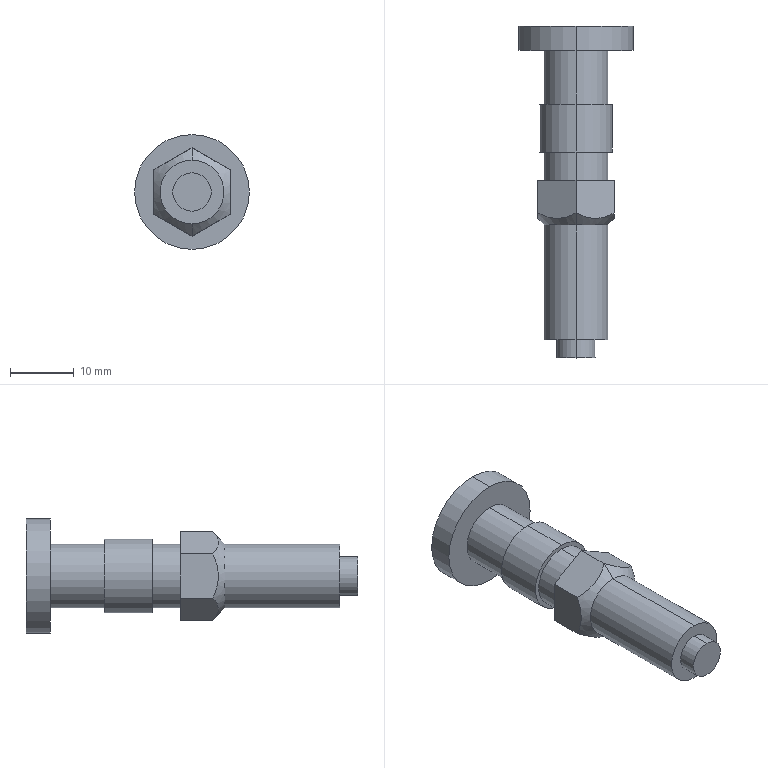Part | STEP file | Knob plunger PMXYK10 | 1 solid | 27 faces | box 18 x 52 x 18 mm | volume 5094 mm3 | plane 13 | cylinder 12 | cone 2 | commonest cylinder face diameters 10 x6 6 x2 11.5 x2 18 x2